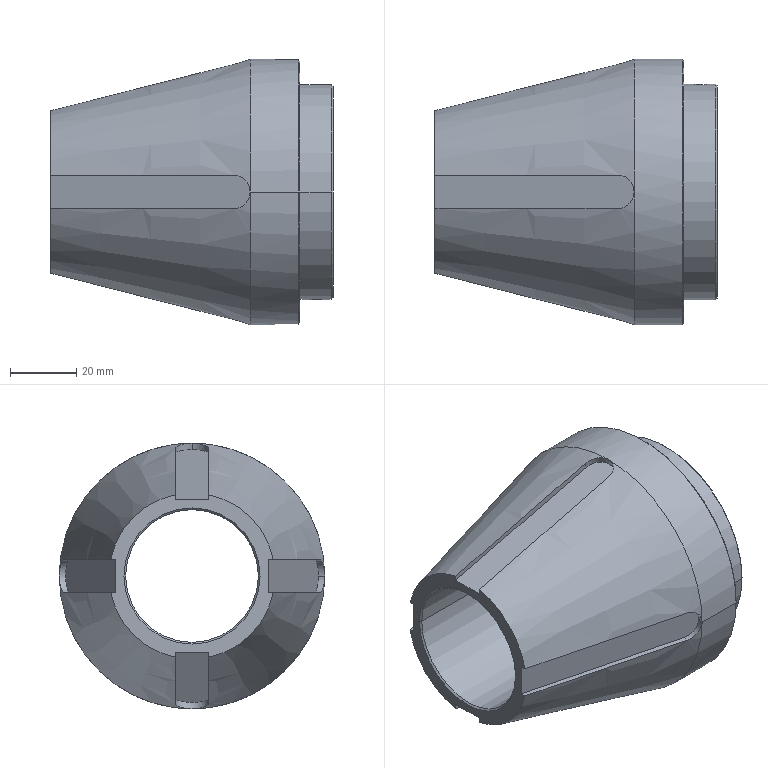Part | STEP file | Coil positioning piece 2 | 1 solid | 47 faces | box 85 x 80 x 80 mm | volume 199257 mm3 | cylinder 16 | plane 15 | cone 12 | spline 4 | commonest cylinder face diameters 10 x6 4.917 x4 40 x2 65 x2 80 x2